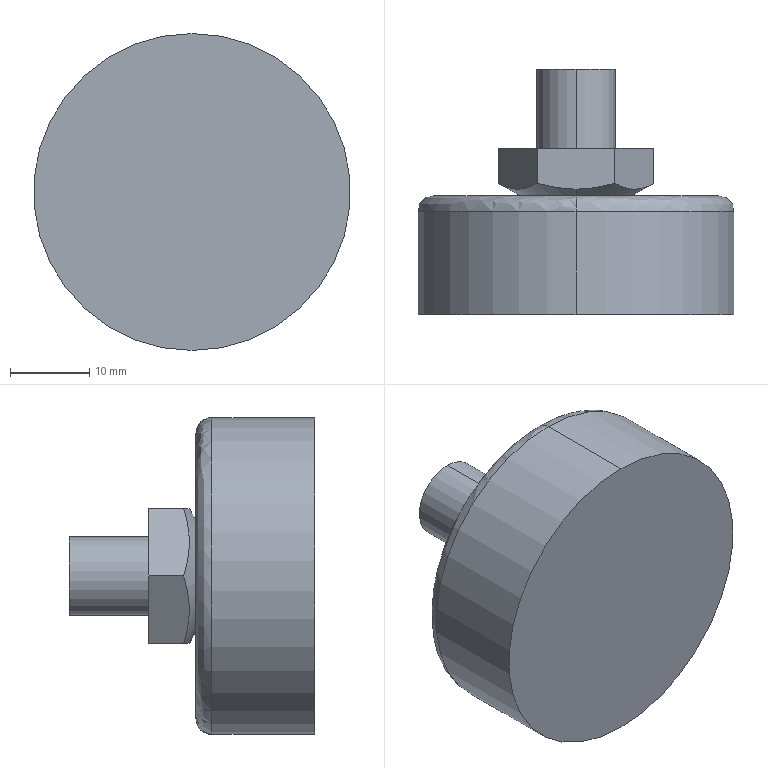Part | STEP file | _pad240-10-30pad2 | 1 solid | 24 faces | box 40 x 31 x 40 mm | volume 20949 mm3 | plane 12 | cylinder 8 | spline 2 | cone 2 | commonest cylinder face diameters 10 x2 17 x2 25 x2 40 x2